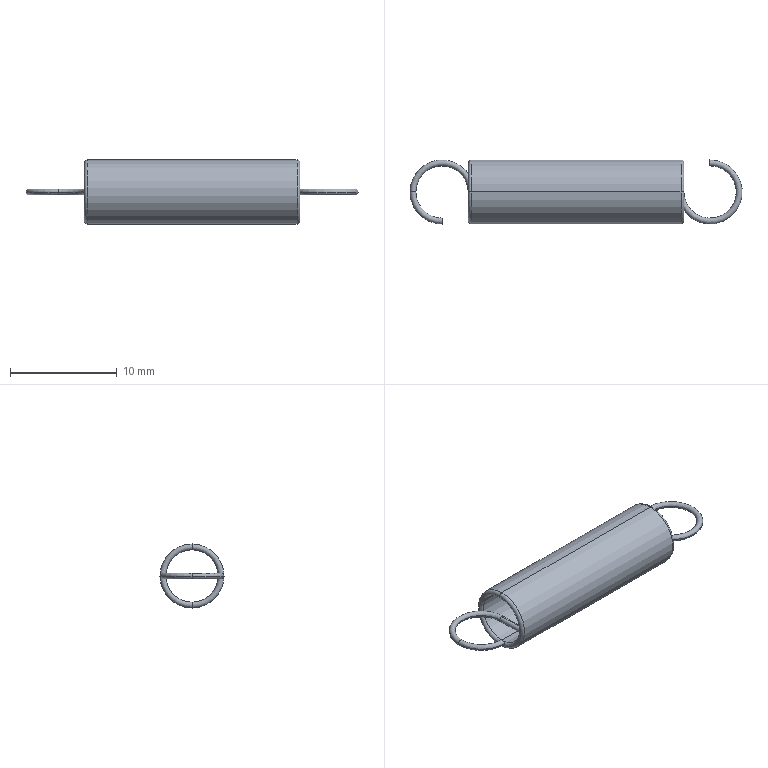Part | STEP file | AWA6_30_AWA6-30 | 1 solid | 20 faces | box 31.1 x 6 x 6 mm | volume 196.407 mm3 | torus 10 | cylinder 8 | plane 2 | commonest cylinder face diameters 0.55 x4 4.9 x2 6 x2